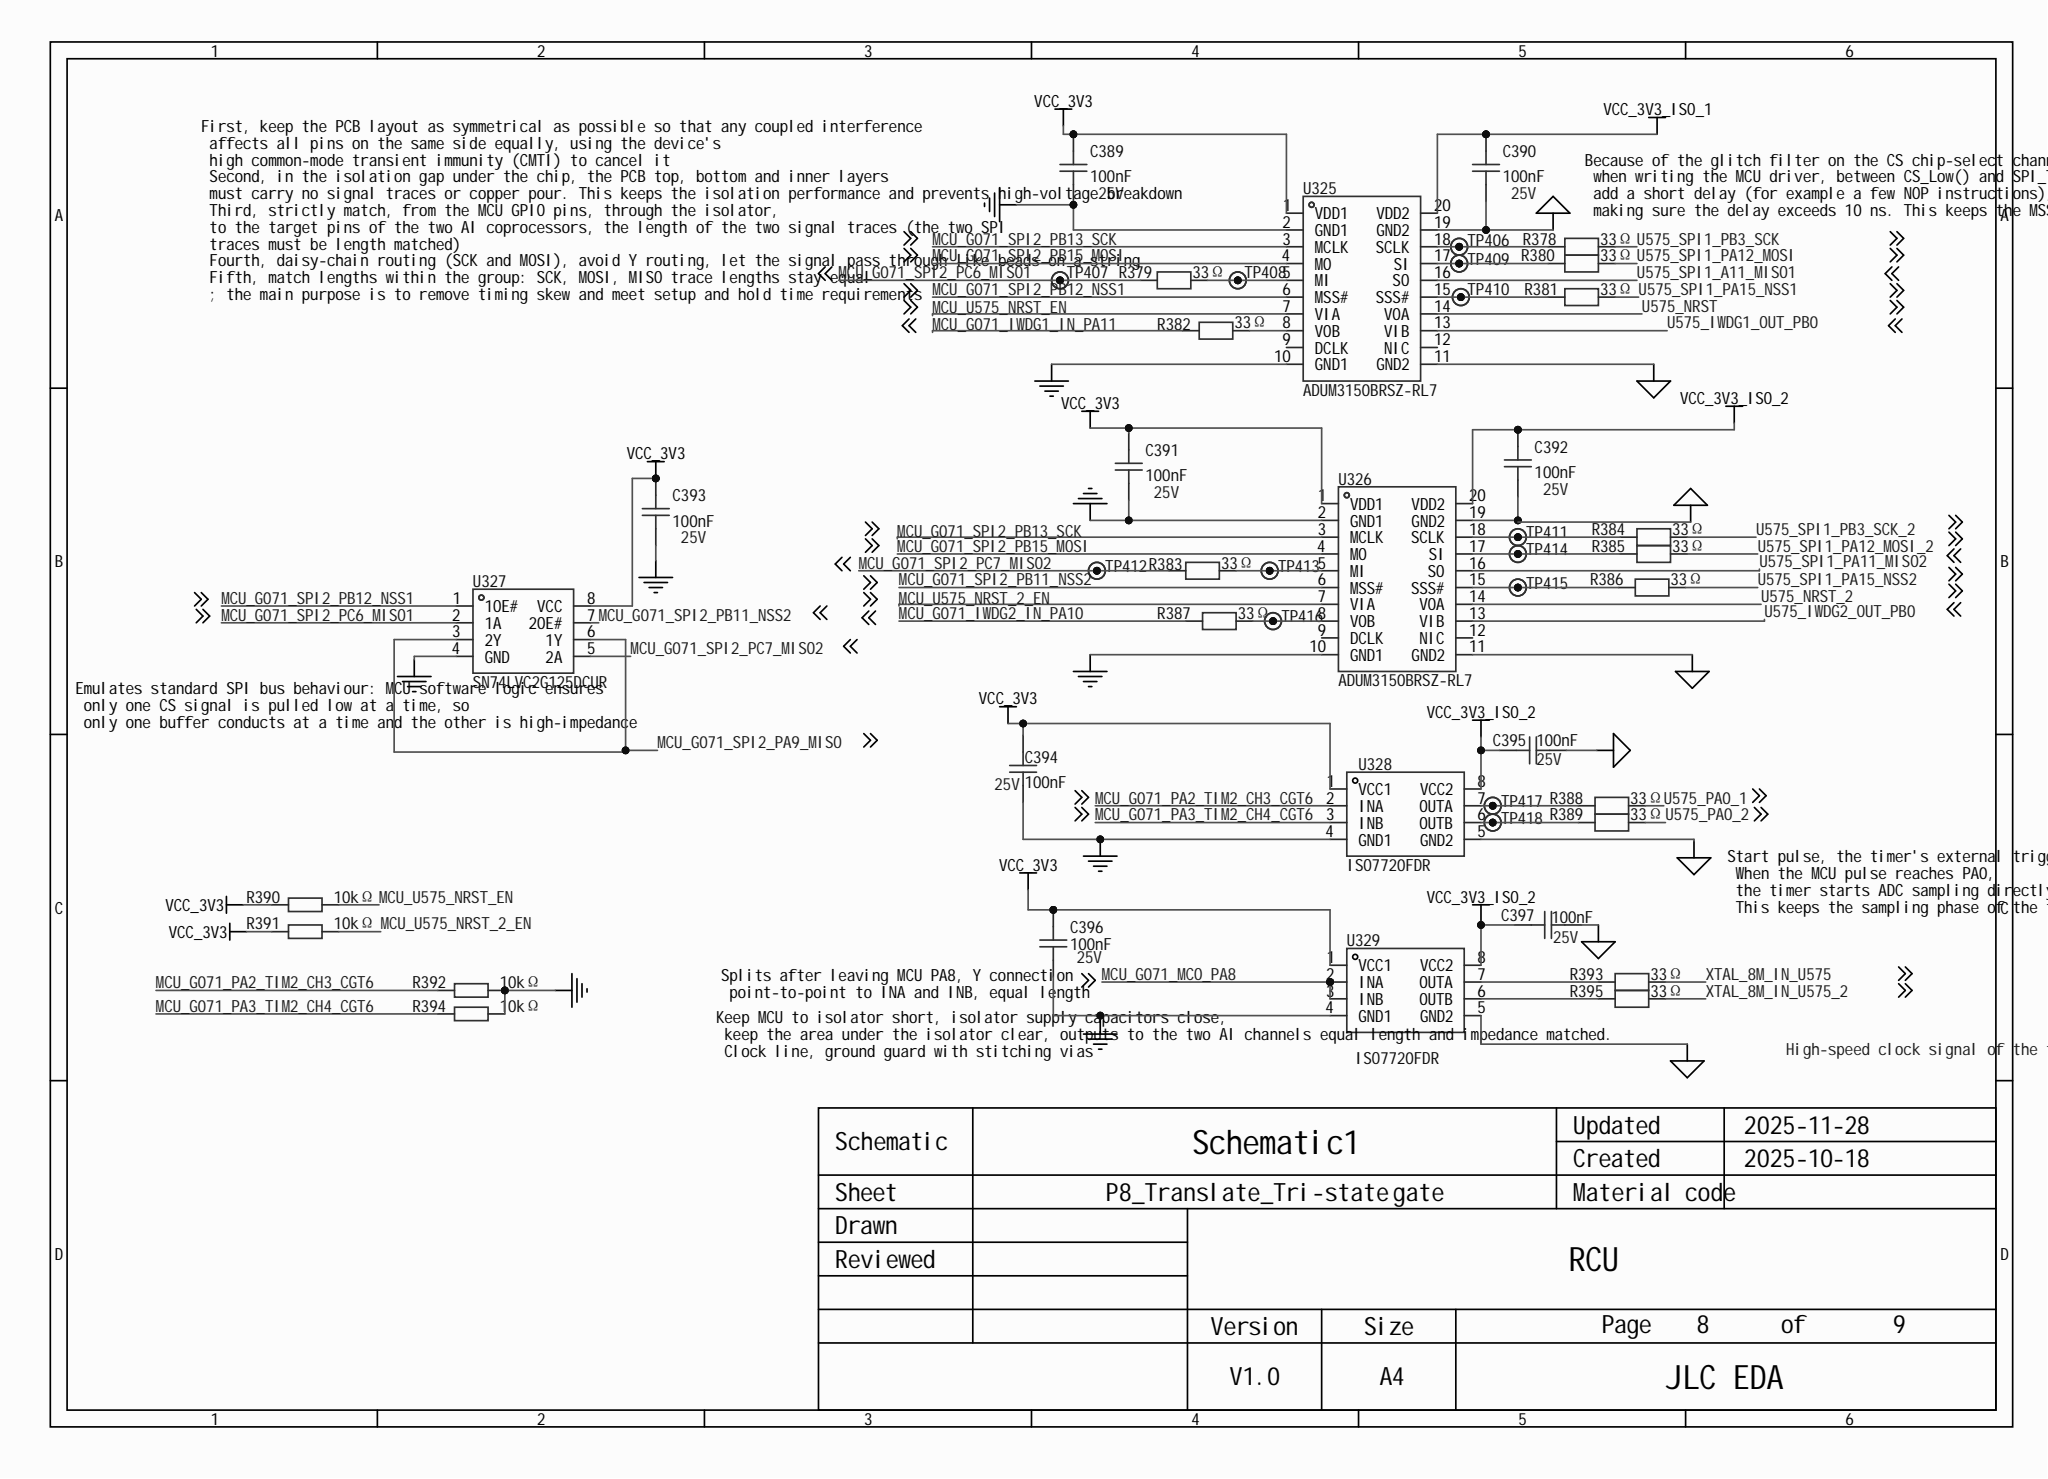Circuit board | Altium Designer | 424 parts | 202 nets | one sheet of the schematic
Parts on this sheet (reference | value | footprint):
C389 | 100nF | C0603
C390 | 100nF | C0603
C391 | 100nF | C0603
C392 | 100nF | C0603
C393 | 100nF | C0603
C394 | 100nF | C0603
C395 | 100nF | C0603
C396 | 100nF | C0603
C397 | 100nF | C0603
R378 | 33Ω | R0603
R379 | 33Ω | R0603
R380 | 33Ω | R0603
R381 | 33Ω | R0603
R382 | 33Ω | R0603
R383 | 33Ω | R0603
R384 | 33Ω | R0603
R385 | 33Ω | R0603
R386 | 33Ω | R0603
R387 | 33Ω | R0603
R388 | 33Ω | R0603
R389 | 33Ω | R0603
R390 | 10kΩ | R0603
R391 | 10kΩ | R0603
R392 | 10kΩ | R0603
R393 | 33Ω | R0603
R394 | 10kΩ | R0603
R395 | 33Ω | R0603
TP406 | Test-Point-0.5mm
TP407 | Test-Point-0.5mm
TP408 | Test-Point-0.5mm
TP409 | Test-Point-0.5mm
TP410 | Test-Point-0.5mm
TP411 | Test-Point-0.5mm
TP412 | Test-Point-0.5mm
TP413 | Test-Point-0.5mm
TP414 | Test-Point-0.5mm
TP415 | Test-Point-0.5mm
TP416 | Test-Point-0.5mm
TP417 | Test-Point-0.5mm
TP418 | Test-Point-0.5mm
U325 | ADUM3150BRSZ-RL7 | SSOP-20_L7.2-W5.3-P0.65-LS7.8-BL
U326 | ADUM3150BRSZ-RL7 | SSOP-20_L7.2-W5.3-P0.65-LS7.8-BL
U327 | SN74LVC2G125DCUR | VSON8_L2.0-W2.3-P0.50-LS3.1-BL
U328 | ISO7720FDR | SOIC-8_L5.0-W4.0-P1.27-LS6.1-BL
U329 | ISO7720FDR | SOIC-8_L5.0-W4.0-P1.27-LS6.1-BL
Nets of these parts (net: part-pin ...):
XTAL_8M_IN_U575_2: R395-1
XTAL_8M_IN_U575: R393-1
VCC_3V3_ISO_2: C392-1 C395-1 C397-1 U326-20 U328-8 U329-8
VCC_3V3_ISO_1: C390-1 U325-20
VCC_3V3: C389-1 C391-1 C393-1 C394-1 C396-1 R390-1 R391-1 U325-1 U326-1 U327-8 U328-1 U329-1
U575_SPI1_PB3_SCK_2: R384-1
U575_SPI1_PB3_SCK: R378-1
U575_SPI1_PA15_NSS2: R386-1
U575_SPI1_PA15_NSS1: R381-1
U575_SPI1_PA12_MOSI_2: R385-1
U575_SPI1_PA12_MOSI: R380-1
U575_SPI1_PA11_MISO2: U326-16
U575_SPI1_A11_MISO1: U325-16
U575_PA0_2: R389-1
U575_PA0_1: R388-1
U575_NRST_2: U326-14
U575_NRST: U325-14
U575_IWDG2_OUT_PB0: U326-13
U575_IWDG1_OUT_PB0: U325-13
PGND: C390-2 C392-2 C395-2 C397-2 U325-11 U325-19 U326-11 U326-19 U328-5 U329-5
NetR395_2: R395-2 U329-6
NetR393_2: R393-2 U329-7
NetR389_2: R389-2 TP418-1 U328-6
NetR388_2: R388-2 TP417-1 U328-7
NetR387_1: R387-1 TP416-1 U326-8
NetR386_2: R386-2 TP415-1 U326-15
NetR385_2: R385-2 TP414-1 U326-17
NetR384_2: R384-2 TP411-1 U326-18
NetR383_1: R383-1 TP413-1 U326-5
NetR382_1: R382-1 U325-8
NetR381_2: R381-2 TP410-1 U325-15
NetR380_2: R380-2 TP409-1 U325-17
NetR379_1: R379-1 TP408-1 U325-5
NetR378_2: R378-2 TP406-1 U325-18
MCU_U575_NRST_EN: R390-2 U325-7
MCU_U575_NRST_2_EN: R391-2 U326-7
MCU_G071_SPI2_PC7_MISO2: R383-2 TP412-1 U327-5
MCU_G071_SPI2_PC6_MISO1: R379-2 TP407-1 U327-2
MCU_G071_SPI2_PB15_MOSI: U325-4 U326-4
MCU_G071_SPI2_PB13_SCK: U325-3 U326-3
MCU_G071_SPI2_PB12_NSS1: U325-6 U327-1
MCU_G071_SPI2_PB11_NSS2: U326-6 U327-7
MCU_G071_SPI2_PA9_MISO: U327-3 U327-6
MCU_G071_PA3_TIM2_CH4_CGT6: R394-1 U328-3
MCU_G071_PA2_TIM2_CH3_CGT6: R392-1 U328-2
MCU_G071_MCO_PA8: U329-2 U329-3
MCU_G071_IWDG2_IN_PA10: R387-2
MCU_G071_IWDG1_IN_PA11: R382-2
GND: C389-2 C391-2 C393-2 C394-2 C396-2 R392-2 R394-2 U325-2 U325-10 U326-2 U326-10 U327-4 U328-4 U329-4